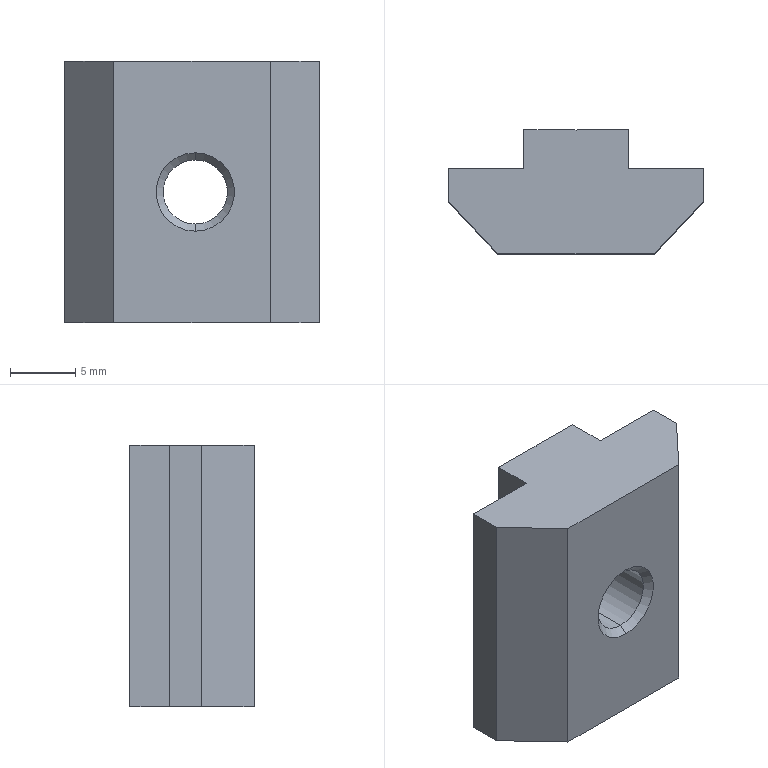Part | SolidWorks | features BaseBody 1 | 1 solid | 23 faces | box 19.5 x 9.5 x 20 mm | volume 2530 mm3 | plane 17 | cone 4 | cylinder 2 | commonest cylinder face diameters 4.917 x2
STEP:
#1=CARTESIAN_POINT('',(10.,0.5415,-7.542));
#2=VERTEX_POINT('',#1);
#3=CARTESIAN_POINT('',(10.,0.5415,-12.458));
#4=VERTEX_POINT('',#3);
#5=CARTESIAN_POINT('',(10.,0.5415,-10.));
#6=DIRECTION('',(0.,-1.,0.));
#7=DIRECTION('',(0.,0.,-1.));
#8=AXIS2_PLACEMENT_3D('',#5,#6,#7);
#9=CIRCLE('',#8,2.458);
#10=EDGE_CURVE('',#2,#4,#9,.T.);
#11=ORIENTED_EDGE('',*,*,#10,.F.);
#12=CARTESIAN_POINT('',(10.,0.,-7.));
#13=VERTEX_POINT('',#12);
#14=CARTESIAN_POINT('',(10.,0.,-7.));
#15=DIRECTION('',(0.,-0.7071,0.7071));
#16=VECTOR('',#15,1000.);
#17=LINE('',#14,#16);
#18=EDGE_CURVE('',#2,#13,#17,.T.);
#19=ORIENTED_EDGE('',*,*,#18,.T.);
#20=CARTESIAN_POINT('',(10.,0.,-13.));
#21=VERTEX_POINT('',#20);
#22=CARTESIAN_POINT('',(10.,0.,-10.));
#23=DIRECTION('',(0.,1.,0.));
#24=DIRECTION('',(0.,0.,-1.));
#25=AXIS2_PLACEMENT_3D('',#22,#23,#24);
#26=CIRCLE('',#25,3.);
#27=EDGE_CURVE('',#21,#13,#26,.T.);
#28=ORIENTED_EDGE('',*,*,#27,.F.);
#29=CARTESIAN_POINT('',(10.,0.,-13.));
#30=DIRECTION('',(0.,-0.7071,-0.7071));
#31=VECTOR('',#30,1000.);
#32=LINE('',#29,#31);
#33=EDGE_CURVE('',#4,#21,#32,.T.);
#34=ORIENTED_EDGE('',*,*,#33,.F.);
#35=EDGE_LOOP('',(#11,#19,#28,#34));
#36=FACE_OUTER_BOUND('',#35,.T.);
#37=CARTESIAN_POINT('',(10.,0.,-10.));
#38=DIRECTION('',(0.,-1.,0.));
#39=DIRECTION('',(0.,0.,-1.));
#40=AXIS2_PLACEMENT_3D('',#37,#38,#39);
#41=CONICAL_SURFACE('',#40,3.,0.7854);
#42=ADVANCED_FACE('',(#36),#41,.F.);
#43=ORIENTED_EDGE('',*,*,#10,.T.);
#44=CARTESIAN_POINT('',(10.,8.959,-12.459));
#45=VERTEX_POINT('',#44);
#46=CARTESIAN_POINT('',(10.,0.,-12.459));
#47=DIRECTION('',(0.,1.,0.));
#48=VECTOR('',#47,1000.);
#49=LINE('',#46,#48);
#50=EDGE_CURVE('',#4,#45,#49,.T.);
#51=ORIENTED_EDGE('',*,*,#50,.T.);
#52=CARTESIAN_POINT('',(10.,8.959,-7.542));
#53=VERTEX_POINT('',#52);
#54=CARTESIAN_POINT('',(10.,8.959,-10.));
#55=DIRECTION('',(0.,-1.,0.));
#56=DIRECTION('',(0.,0.,1.));
#57=AXIS2_PLACEMENT_3D('',#54,#55,#56);
#58=CIRCLE('',#57,2.458);
#59=EDGE_CURVE('',#53,#45,#58,.T.);
#60=ORIENTED_EDGE('',*,*,#59,.F.);
#61=CARTESIAN_POINT('',(10.,0.,-7.542));
#62=DIRECTION('',(0.,1.,0.));
#63=VECTOR('',#62,1000.);
#64=LINE('',#61,#63);
#65=EDGE_CURVE('',#2,#53,#64,.T.);
#66=ORIENTED_EDGE('',*,*,#65,.F.);
#67=EDGE_LOOP('',(#43,#51,#60,#66));
#68=FACE_OUTER_BOUND('',#67,.T.);
#69=CARTESIAN_POINT('',(10.,0.,-10.));
#70=DIRECTION('',(0.,1.,0.));
#71=DIRECTION('',(0.,0.,1.));
#72=AXIS2_PLACEMENT_3D('',#69,#70,#71);
#73=CYLINDRICAL_SURFACE('',#72,2.458);
#74=ADVANCED_FACE('',(#68),#73,.F.);
#75=ORIENTED_EDGE('',*,*,#59,.T.);
#76=CARTESIAN_POINT('',(10.,9.5,-13.));
#77=VERTEX_POINT('',#76);
#78=CARTESIAN_POINT('',(10.,9.5,-13.));
#79=DIRECTION('',(0.,0.7071,-0.7071));
#80=VECTOR('',#79,1000.);
#81=LINE('',#78,#80);
#82=EDGE_CURVE('',#45,#77,#81,.T.);
#83=ORIENTED_EDGE('',*,*,#82,.T.);
#84=CARTESIAN_POINT('',(9.85,9.5,-12.996));
#85=VERTEX_POINT('',#84);
#86=CARTESIAN_POINT('',(10.,9.5,-10.));
#87=DIRECTION('',(0.,-1.,0.));
#88=DIRECTION('',(0.,0.,1.));
#89=AXIS2_PLACEMENT_3D('',#86,#87,#88);
#90=CIRCLE('',#89,3.);
#91=EDGE_CURVE('',#85,#77,#90,.T.);
#92=ORIENTED_EDGE('',*,*,#91,.F.);
#93=CARTESIAN_POINT('',(9.75,9.42,-12.909));
#94=VERTEX_POINT('',#93);
#95=CARTESIAN_POINT('',(9.75,9.42,-12.909));
#96=CARTESIAN_POINT('',(9.783,9.446,-12.938));
#97=CARTESIAN_POINT('',(9.816,9.473,-12.967));
#98=CARTESIAN_POINT('',(9.85,9.5,-12.996));
#99=(BOUNDED_CURVE()B_SPLINE_CURVE(3,(#95,#96,#97,#98),.UNSPECIFIED.,.F.,.F.)B_SPLINE_CURVE_WITH_KNOTS((4,4),(3.735,3.756),.UNSPECIFIED.)CURVE()GEOMETRIC_REPRESENTATION_ITEM()RATIONAL_B_SPLINE_CURVE((1.,1.,1.,1.))REPRESENTATION_ITEM(''));
#100=EDGE_CURVE('',#94,#85,#99,.T.);
#101=ORIENTED_EDGE('',*,*,#100,.F.);
#102=CARTESIAN_POINT('',(9.65,9.5,-12.98));
#103=VERTEX_POINT('',#102);
#104=CARTESIAN_POINT('',(9.65,9.5,-12.98));
#105=CARTESIAN_POINT('',(9.684,9.473,-12.956));
#106=CARTESIAN_POINT('',(9.717,9.446,-12.933));
#107=CARTESIAN_POINT('',(9.75,9.42,-12.909));
#108=(BOUNDED_CURVE()B_SPLINE_CURVE(3,(#104,#105,#106,#107),.UNSPECIFIED.,.F.,.F.)B_SPLINE_CURVE_WITH_KNOTS((4,4),(2.424,2.445),.UNSPECIFIED.)CURVE()GEOMETRIC_REPRESENTATION_ITEM()RATIONAL_B_SPLINE_CURVE((1.,1.,1.,1.))REPRESENTATION_ITEM(''));
#109=EDGE_CURVE('',#103,#94,#108,.T.);
#110=ORIENTED_EDGE('',*,*,#109,.F.);
#111=CARTESIAN_POINT('',(9.65,9.5,-7.02));
#112=VERTEX_POINT('',#111);
#113=CARTESIAN_POINT('',(10.,9.5,-10.));
#114=DIRECTION('',(0.,-1.,0.));
#115=DIRECTION('',(0.,0.,1.));
#116=AXIS2_PLACEMENT_3D('',#113,#114,#115);
#117=CIRCLE('',#116,3.);
#118=EDGE_CURVE('',#112,#103,#117,.T.);
#119=ORIENTED_EDGE('',*,*,#118,.F.);
#120=CARTESIAN_POINT('',(9.75,9.42,-7.091));
#121=VERTEX_POINT('',#120);
#122=CARTESIAN_POINT('',(9.75,9.42,-7.091));
#123=CARTESIAN_POINT('',(9.717,9.446,-7.067));
#124=CARTESIAN_POINT('',(9.684,9.473,-7.044));
#125=CARTESIAN_POINT('',(9.65,9.5,-7.02));
#126=(BOUNDED_CURVE()B_SPLINE_CURVE(3,(#122,#123,#124,#125),.UNSPECIFIED.,.F.,.F.)B_SPLINE_CURVE_WITH_KNOTS((4,4),(3.838,3.859),.UNSPECIFIED.)CURVE()GEOMETRIC_REPRESENTATION_ITEM()RATIONAL_B_SPLINE_CURVE((1.,1.,1.,1.))REPRESENTATION_ITEM(''));
#127=EDGE_CURVE('',#121,#112,#126,.T.);
#128=ORIENTED_EDGE('',*,*,#127,.F.);
#129=CARTESIAN_POINT('',(9.85,9.5,-7.004));
#130=VERTEX_POINT('',#129);
#131=CARTESIAN_POINT('',(9.85,9.5,-7.004));
#132=CARTESIAN_POINT('',(9.816,9.473,-7.033));
#133=CARTESIAN_POINT('',(9.783,9.446,-7.062));
#134=CARTESIAN_POINT('',(9.75,9.42,-7.091));
#135=(BOUNDED_CURVE()B_SPLINE_CURVE(3,(#131,#132,#133,#134),.UNSPECIFIED.,.F.,.F.)B_SPLINE_CURVE_WITH_KNOTS((4,4),(2.528,2.548),.UNSPECIFIED.)CURVE()GEOMETRIC_REPRESENTATION_ITEM()RATIONAL_B_SPLINE_CURVE((1.,1.,1.,1.))REPRESENTATION_ITEM(''));
#136=EDGE_CURVE('',#130,#121,#135,.T.);
#137=ORIENTED_EDGE('',*,*,#136,.F.);
#138=CARTESIAN_POINT('',(10.,9.5,-7.));
#139=VERTEX_POINT('',#138);
#140=CARTESIAN_POINT('',(10.,9.5,-10.));
#141=DIRECTION('',(0.,-1.,0.));
#142=DIRECTION('',(0.,0.,1.));
#143=AXIS2_PLACEMENT_3D('',#140,#141,#142);
#144=CIRCLE('',#143,3.);
#145=EDGE_CURVE('',#139,#130,#144,.T.);
#146=ORIENTED_EDGE('',*,*,#145,.F.);
#147=CARTESIAN_POINT('',(10.,9.5,-7.));
#148=DIRECTION('',(0.,0.7071,0.7071));
#149=VECTOR('',#148,1000.);
#150=LINE('',#147,#149);
#151=EDGE_CURVE('',#53,#139,#150,.T.);
#152=ORIENTED_EDGE('',*,*,#151,.F.);
#153=EDGE_LOOP('',(#75,#83,#92,#101,#110,#119,#128,#137,#146,#152));
#154=FACE_OUTER_BOUND('',#153,.T.);
#155=CARTESIAN_POINT('',(10.,9.5,-10.));
#156=DIRECTION('',(0.,1.,0.));
#157=DIRECTION('',(0.,0.,1.));
#158=AXIS2_PLACEMENT_3D('',#155,#156,#157);
#159=CONICAL_SURFACE('',#158,3.,0.7854);
#160=ADVANCED_FACE('',(#154),#159,.F.);
#161=CARTESIAN_POINT('',(15.75,0.,0.));
#162=VERTEX_POINT('',#161);
#163=CARTESIAN_POINT('',(3.75,0.,0.));
#164=VERTEX_POINT('',#163);
#165=CARTESIAN_POINT('',(3.75,0.,0.));
#166=DIRECTION('',(-1.,0.,0.));
#167=VECTOR('',#166,1000.);
#168=LINE('',#165,#167);
#169=EDGE_CURVE('',#162,#164,#168,.T.);
#170=ORIENTED_EDGE('',*,*,#169,.T.);
#171=CARTESIAN_POINT('',(3.75,0.,-20.));
#172=VERTEX_POINT('',#171);
#173=CARTESIAN_POINT('',(3.75,0.,-20.));
#174=DIRECTION('',(0.,0.,-1.));
#175=VECTOR('',#174,1000.);
#176=LINE('',#173,#175);
#177=EDGE_CURVE('',#164,#172,#176,.T.);
#178=ORIENTED_EDGE('',*,*,#177,.T.);
#179=CARTESIAN_POINT('',(15.75,0.,-20.));
#180=VERTEX_POINT('',#179);
#181=CARTESIAN_POINT('',(3.75,0.,-20.));
#182=DIRECTION('',(1.,0.,0.));
#183=VECTOR('',#182,1000.);
#184=LINE('',#181,#183);
#185=EDGE_CURVE('',#172,#180,#184,.T.);
#186=ORIENTED_EDGE('',*,*,#185,.T.);
#187=CARTESIAN_POINT('',(15.75,0.,-20.));
#188=DIRECTION('',(0.,0.,1.));
#189=VECTOR('',#188,1000.);
#190=LINE('',#187,#189);
#191=EDGE_CURVE('',#180,#162,#190,.T.);
#192=ORIENTED_EDGE('',*,*,#191,.T.);
#193=EDGE_LOOP('',(#170,#178,#186,#192));
#194=FACE_OUTER_BOUND('',#193,.T.);
#195=ORIENTED_EDGE('',*,*,#27,.T.);
#196=CARTESIAN_POINT('',(10.,0.,-10.));
#197=DIRECTION('',(0.,1.,0.));
#198=DIRECTION('',(0.,0.,-1.));
#199=AXIS2_PLACEMENT_3D('',#196,#197,#198);
#200=CIRCLE('',#199,3.);
#201=EDGE_CURVE('',#13,#21,#200,.T.);
#202=ORIENTED_EDGE('',*,*,#201,.T.);
#203=EDGE_LOOP('',(#195,#202));
#204=FACE_BOUND('',#203,.T.);
#205=CARTESIAN_POINT('',(3.75,0.,-20.));
#206=DIRECTION('',(0.,-1.,0.));
#207=DIRECTION('',(0.,0.,-1.));
#208=AXIS2_PLACEMENT_3D('',#205,#206,#207);
#209=PLANE('',#208);
#210=ADVANCED_FACE('',(#194,#204),#209,.T.);
#211=CARTESIAN_POINT('',(0.,4.,0.));
#212=VERTEX_POINT('',#211);
#213=CARTESIAN_POINT('',(0.,4.,0.));
#214=DIRECTION('',(-0.6839,0.7295,0.));
#215=VECTOR('',#214,1000.);
#216=LINE('',#213,#215);
#217=EDGE_CURVE('',#164,#212,#216,.T.);
#218=ORIENTED_EDGE('',*,*,#217,.T.);
#219=CARTESIAN_POINT('',(0.,4.,-20.));
#220=VERTEX_POINT('',#219);
#221=CARTESIAN_POINT('',(0.,4.,-20.));
#222=DIRECTION('',(0.,0.,-1.));
#223=VECTOR('',#222,1000.);
#224=LINE('',#221,#223);
#225=EDGE_CURVE('',#212,#220,#224,.T.);
#226=ORIENTED_EDGE('',*,*,#225,.T.);
#227=CARTESIAN_POINT('',(0.,4.,-20.));
#228=DIRECTION('',(0.6839,-0.7295,0.));
#229=VECTOR('',#228,1000.);
#230=LINE('',#227,#229);
#231=EDGE_CURVE('',#220,#172,#230,.T.);
#232=ORIENTED_EDGE('',*,*,#231,.T.);
#233=ORIENTED_EDGE('',*,*,#177,.F.);
#234=EDGE_LOOP('',(#218,#226,#232,#233));
#235=FACE_OUTER_BOUND('',#234,.T.);
#236=CARTESIAN_POINT('',(0.,4.,-20.));
#237=DIRECTION('',(-0.7295,-0.6839,0.));
#238=DIRECTION('',(0.6839,-0.7295,0.));
#239=AXIS2_PLACEMENT_3D('',#236,#237,#238);
#240=PLANE('',#239);
#241=ADVANCED_FACE('',(#235),#240,.T.);
#242=CARTESIAN_POINT('',(9.75,9.42,0.));
#243=VERTEX_POINT('',#242);
#244=CARTESIAN_POINT('',(9.85,9.5,0.));
#245=VERTEX_POINT('',#244);
#246=CARTESIAN_POINT('',(9.85,9.5,0.));
#247=DIRECTION('',(0.7809,0.6247,0.));
#248=VECTOR('',#247,1000.);
#249=LINE('',#246,#248);
#250=EDGE_CURVE('',#243,#245,#249,.T.);
#251=ORIENTED_EDGE('',*,*,#250,.F.);
#252=CARTESIAN_POINT('',(9.65,9.5,0.));
#253=VERTEX_POINT('',#252);
#254=CARTESIAN_POINT('',(9.75,9.42,0.));
#255=DIRECTION('',(0.7809,-0.6247,0.));
#256=VECTOR('',#255,1000.);
#257=LINE('',#254,#256);
#258=EDGE_CURVE('',#253,#243,#257,.T.);
#259=ORIENTED_EDGE('',*,*,#258,.F.);
#260=CARTESIAN_POINT('',(5.75,9.5,0.));
#261=VERTEX_POINT('',#260);
#262=CARTESIAN_POINT('',(0.,9.5,0.));
#263=DIRECTION('',(-1.,0.,0.));
#264=VECTOR('',#263,1000.);
#265=LINE('',#262,#264);
#266=EDGE_CURVE('',#253,#261,#265,.T.);
#267=ORIENTED_EDGE('',*,*,#266,.T.);
#268=CARTESIAN_POINT('',(5.75,6.5,0.));
#269=VERTEX_POINT('',#268);
#270=CARTESIAN_POINT('',(5.75,0.,0.));
#271=DIRECTION('',(0.,-1.,0.));
#272=VECTOR('',#271,1000.);
#273=LINE('',#270,#272);
#274=EDGE_CURVE('',#261,#269,#273,.T.);
#275=ORIENTED_EDGE('',*,*,#274,.T.);
#276=CARTESIAN_POINT('',(0.,6.5,0.));
#277=VERTEX_POINT('',#276);
#278=CARTESIAN_POINT('',(0.,6.5,0.));
#279=DIRECTION('',(-1.,0.,0.));
#280=VECTOR('',#279,1000.);
#281=LINE('',#278,#280);
#282=EDGE_CURVE('',#269,#277,#281,.T.);
#283=ORIENTED_EDGE('',*,*,#282,.T.);
#284=CARTESIAN_POINT('',(0.,0.,0.));
#285=DIRECTION('',(0.,-1.,0.));
#286=VECTOR('',#285,1000.);
#287=LINE('',#284,#286);
#288=EDGE_CURVE('',#277,#212,#287,.T.);
#289=ORIENTED_EDGE('',*,*,#288,.T.);
#290=ORIENTED_EDGE('',*,*,#217,.F.);
#291=ORIENTED_EDGE('',*,*,#169,.F.);
#292=CARTESIAN_POINT('',(19.5,4.,0.));
#293=VERTEX_POINT('',#292);
#294=CARTESIAN_POINT('',(15.75,0.,0.));
#295=DIRECTION('',(0.6839,0.7295,0.));
#296=VECTOR('',#295,1000.);
#297=LINE('',#294,#296);
#298=EDGE_CURVE('',#162,#293,#297,.T.);
#299=ORIENTED_EDGE('',*,*,#298,.T.);
#300=CARTESIAN_POINT('',(19.5,6.5,0.));
#301=VERTEX_POINT('',#300);
#302=CARTESIAN_POINT('',(19.5,0.,0.));
#303=DIRECTION('',(0.,1.,0.));
#304=VECTOR('',#303,1000.);
#305=LINE('',#302,#304);
#306=EDGE_CURVE('',#293,#301,#305,.T.);
#307=ORIENTED_EDGE('',*,*,#306,.T.);
#308=CARTESIAN_POINT('',(13.75,6.5,0.));
#309=VERTEX_POINT('',#308);
#310=CARTESIAN_POINT('',(0.,6.5,0.));
#311=DIRECTION('',(-1.,0.,0.));
#312=VECTOR('',#311,1000.);
#313=LINE('',#310,#312);
#314=EDGE_CURVE('',#301,#309,#313,.T.);
#315=ORIENTED_EDGE('',*,*,#314,.T.);
#316=CARTESIAN_POINT('',(13.75,9.5,0.));
#317=VERTEX_POINT('',#316);
#318=CARTESIAN_POINT('',(13.75,0.,0.));
#319=DIRECTION('',(0.,1.,0.));
#320=VECTOR('',#319,1000.);
#321=LINE('',#318,#320);
#322=EDGE_CURVE('',#309,#317,#321,.T.);
#323=ORIENTED_EDGE('',*,*,#322,.T.);
#324=CARTESIAN_POINT('',(0.,9.5,0.));
#325=DIRECTION('',(-1.,0.,0.));
#326=VECTOR('',#325,1000.);
#327=LINE('',#324,#326);
#328=EDGE_CURVE('',#317,#245,#327,.T.);
#329=ORIENTED_EDGE('',*,*,#328,.T.);
#330=EDGE_LOOP('',(#251,#259,#267,#275,#283,#289,#290,#291,#299,#307,#315,#323,#329));
#331=FACE_OUTER_BOUND('',#330,.T.);
#332=CARTESIAN_POINT('',(0.,0.,0.));
#333=DIRECTION('',(0.,0.,1.));
#334=DIRECTION('',(1.,0.,0.));
#335=AXIS2_PLACEMENT_3D('',#332,#333,#334);
#336=PLANE('',#335);
#337=ADVANCED_FACE('',(#331),#336,.T.);
#338=ORIENTED_EDGE('',*,*,#298,.F.);
#339=ORIENTED_EDGE('',*,*,#191,.F.);
#340=CARTESIAN_POINT('',(19.5,4.,-20.));
#341=VERTEX_POINT('',#340);
#342=CARTESIAN_POINT('',(15.75,0.,-20.));
#343=DIRECTION('',(0.6839,0.7295,0.));
#344=VECTOR('',#343,1000.);
#345=LINE('',#342,#344);
#346=EDGE_CURVE('',#180,#341,#345,.T.);
#347=ORIENTED_EDGE('',*,*,#346,.T.);
#348=CARTESIAN_POINT('',(19.5,4.,-20.));
#349=DIRECTION('',(0.,0.,1.));
#350=VECTOR('',#349,1000.);
#351=LINE('',#348,#350);
#352=EDGE_CURVE('',#341,#293,#351,.T.);
#353=ORIENTED_EDGE('',*,*,#352,.T.);
#354=EDGE_LOOP('',(#338,#339,#347,#353));
#355=FACE_OUTER_BOUND('',#354,.T.);
#356=CARTESIAN_POINT('',(15.75,0.,-20.));
#357=DIRECTION('',(0.7295,-0.6839,0.));
#358=DIRECTION('',(0.6839,0.7295,0.));
#359=AXIS2_PLACEMENT_3D('',#356,#357,#358);
#360=PLANE('',#359);
#361=ADVANCED_FACE('',(#355),#360,.T.);
#362=CARTESIAN_POINT('',(9.65,9.5,-20.));
#363=VERTEX_POINT('',#362);
#364=CARTESIAN_POINT('',(5.75,9.5,-20.));
#365=VERTEX_POINT('',#364);
#366=CARTESIAN_POINT('',(0.,9.5,-20.));
#367=DIRECTION('',(-1.,0.,0.));
#368=VECTOR('',#367,1000.);
#369=LINE('',#366,#368);
#370=EDGE_CURVE('',#363,#365,#369,.T.);
#371=ORIENTED_EDGE('',*,*,#370,.F.);
#372=CARTESIAN_POINT('',(9.75,9.42,-20.));
#373=VERTEX_POINT('',#372);
#374=CARTESIAN_POINT('',(9.75,9.42,-20.));
#375=DIRECTION('',(-0.7809,0.6247,0.));
#376=VECTOR('',#375,1000.);
#377=LINE('',#374,#376);
#378=EDGE_CURVE('',#373,#363,#377,.T.);
#379=ORIENTED_EDGE('',*,*,#378,.F.);
#380=CARTESIAN_POINT('',(9.85,9.5,-20.));
#381=VERTEX_POINT('',#380);
#382=CARTESIAN_POINT('',(9.85,9.5,-20.));
#383=DIRECTION('',(-0.7809,-0.6247,0.));
#384=VECTOR('',#383,1000.);
#385=LINE('',#382,#384);
#386=EDGE_CURVE('',#381,#373,#385,.T.);
#387=ORIENTED_EDGE('',*,*,#386,.F.);
#388=CARTESIAN_POINT('',(13.75,9.5,-20.));
#389=VERTEX_POINT('',#388);
#390=CARTESIAN_POINT('',(0.,9.5,-20.));
#391=DIRECTION('',(-1.,0.,0.));
#392=VECTOR('',#391,1000.);
#393=LINE('',#390,#392);
#394=EDGE_CURVE('',#389,#381,#393,.T.);
#395=ORIENTED_EDGE('',*,*,#394,.F.);
#396=CARTESIAN_POINT('',(13.75,6.5,-20.));
#397=VERTEX_POINT('',#396);
#398=CARTESIAN_POINT('',(13.75,0.,-20.));
#399=DIRECTION('',(0.,1.,0.));
#400=VECTOR('',#399,1000.);
#401=LINE('',#398,#400);
#402=EDGE_CURVE('',#397,#389,#401,.T.);
#403=ORIENTED_EDGE('',*,*,#402,.F.);
#404=CARTESIAN_POINT('',(19.5,6.5,-20.));
#405=VERTEX_POINT('',#404);
#406=CARTESIAN_POINT('',(0.,6.5,-20.));
#407=DIRECTION('',(-1.,0.,0.));
#408=VECTOR('',#407,1000.);
#409=LINE('',#406,#408);
#410=EDGE_CURVE('',#405,#397,#409,.T.);
#411=ORIENTED_EDGE('',*,*,#410,.F.);
#412=CARTESIAN_POINT('',(19.5,0.,-20.));
#413=DIRECTION('',(0.,1.,0.));
#414=VECTOR('',#413,1000.);
#415=LINE('',#412,#414);
#416=EDGE_CURVE('',#341,#405,#415,.T.);
#417=ORIENTED_EDGE('',*,*,#416,.F.);
#418=ORIENTED_EDGE('',*,*,#346,.F.);
#419=ORIENTED_EDGE('',*,*,#185,.F.);
#420=ORIENTED_EDGE('',*,*,#231,.F.);
#421=CARTESIAN_POINT('',(0.,6.5,-20.));
#422=VERTEX_POINT('',#421);
#423=CARTESIAN_POINT('',(0.,0.,-20.));
#424=DIRECTION('',(0.,-1.,0.));
#425=VECTOR('',#424,1000.);
#426=LINE('',#423,#425);
#427=EDGE_CURVE('',#422,#220,#426,.T.);
#428=ORIENTED_EDGE('',*,*,#427,.F.);
#429=CARTESIAN_POINT('',(5.75,6.5,-20.));
#430=VERTEX_POINT('',#429);
#431=CARTESIAN_POINT('',(0.,6.5,-20.));
#432=DIRECTION('',(-1.,0.,0.));
#433=VECTOR('',#432,1000.);
#434=LINE('',#431,#433);
#435=EDGE_CURVE('',#430,#422,#434,.T.);
#436=ORIENTED_EDGE('',*,*,#435,.F.);
#437=CARTESIAN_POINT('',(5.75,0.,-20.));
#438=DIRECTION('',(0.,-1.,0.));
#439=VECTOR('',#438,1000.);
#440=LINE('',#437,#439);
#441=EDGE_CURVE('',#365,#430,#440,.T.);
#442=ORIENTED_EDGE('',*,*,#441,.F.);
#443=EDGE_LOOP('',(#371,#379,#387,#395,#403,#411,#417,#418,#419,#420,#428,#436,#442));
#444=FACE_OUTER_BOUND('',#443,.T.);
#445=CARTESIAN_POINT('',(0.,0.,-20.));
#446=DIRECTION('',(0.,0.,1.));
#447=DIRECTION('',(1.,0.,0.));
#448=AXIS2_PLACEMENT_3D('',#445,#446,#447);
#449=PLANE('',#448);
#450=ADVANCED_FACE('',(#444),#449,.F.);
#451=ORIENTED_EDGE('',*,*,#18,.F.);
#452=CARTESIAN_POINT('',(10.,0.5415,-10.));
#453=DIRECTION('',(0.,-1.,0.));
#454=DIRECTION('',(0.,0.,-1.));
#455=AXIS2_PLACEMENT_3D('',#452,#453,#454);
#456=CIRCLE('',#455,2.458);
#457=EDGE_CURVE('',#4,#2,#456,.T.);
#458=ORIENTED_EDGE('',*,*,#457,.F.);
#459=ORIENTED_EDGE('',*,*,#33,.T.);
#460=ORIENTED_EDGE('',*,*,#201,.F.);
#461=EDGE_LOOP('',(#451,#458,#459,#460));
#462=FACE_OUTER_BOUND('',#461,.T.);
#463=CARTESIAN_POINT('',(10.,0.,-10.));
#464=DIRECTION('',(0.,-1.,0.));
#465=DIRECTION('',(0.,0.,-1.));
#466=AXIS2_PLACEMENT_3D('',#463,#464,#465);
#467=CONICAL_SURFACE('',#466,3.,0.7854);
#468=ADVANCED_FACE('',(#462),#467,.F.);
#469=ORIENTED_EDGE('',*,*,#288,.F.);
#470=CARTESIAN_POINT('',(0.,6.5,-20.));
#471=DIRECTION('',(0.,0.,-1.));
#472=VECTOR('',#471,1000.);
#473=LINE('',#470,#472);
#474=EDGE_CURVE('',#277,#422,#473,.T.);
#475=ORIENTED_EDGE('',*,*,#474,.T.);
#476=ORIENTED_EDGE('',*,*,#427,.T.);
#477=ORIENTED_EDGE('',*,*,#225,.F.);
#478=EDGE_LOOP('',(#469,#475,#476,#477));
#479=FACE_OUTER_BOUND('',#478,.T.);
#480=CARTESIAN_POINT('',(0.,6.5,-20.));
#481=DIRECTION('',(-1.,0.,0.));
#482=DIRECTION('',(0.,0.,1.));
#483=AXIS2_PLACEMENT_3D('',#480,#481,#482);
#484=PLANE('',#483);
#485=ADVANCED_FACE('',(#479),#484,.T.);
#486=ORIENTED_EDGE('',*,*,#328,.F.);
#487=CARTESIAN_POINT('',(13.75,9.5,-20.));
#488=DIRECTION('',(0.,0.,-1.));
#489=VECTOR('',#488,1000.);
#490=LINE('',#487,#489);
#491=EDGE_CURVE('',#317,#389,#490,.T.);
#492=ORIENTED_EDGE('',*,*,#491,.T.);
#493=ORIENTED_EDGE('',*,*,#394,.T.);
#494=CARTESIAN_POINT('',(9.85,9.5,-20.));
#495=DIRECTION('',(0.,0.,1.));
#496=VECTOR('',#495,1000.);
#497=LINE('',#494,#496);
#498=EDGE_CURVE('',#381,#85,#497,.T.);
#499=ORIENTED_EDGE('',*,*,#498,.T.);
#500=ORIENTED_EDGE('',*,*,#91,.T.);
#501=CARTESIAN_POINT('',(10.,9.5,-10.));
#502=DIRECTION('',(0.,-1.,0.));
#503=DIRECTION('',(0.,0.,1.));
#504=AXIS2_PLACEMENT_3D('',#501,#502,#503);
#505=CIRCLE('',#504,3.);
#506=EDGE_CURVE('',#77,#139,#505,.T.);
#507=ORIENTED_EDGE('',*,*,#506,.T.);
#508=ORIENTED_EDGE('',*,*,#145,.T.);
#509=CARTESIAN_POINT('',(9.85,9.5,-20.));
#510=DIRECTION('',(0.,0.,1.));
#511=VECTOR('',#510,1000.);
#512=LINE('',#509,#511);
#513=EDGE_CURVE('',#130,#245,#512,.T.);
#514=ORIENTED_EDGE('',*,*,#513,.T.);
#515=EDGE_LOOP('',(#486,#492,#493,#499,#500,#507,#508,#514));
#516=FACE_OUTER_BOUND('',#515,.T.);
#517=CARTESIAN_POINT('',(13.75,9.5,-20.));
#518=DIRECTION('',(0.,1.,0.));
#519=DIRECTION('',(0.,0.,1.));
#520=AXIS2_PLACEMENT_3D('',#517,#518,#519);
#521=PLANE('',#520);
#522=ADVANCED_FACE('',(#516),#521,.T.);
#523=ORIENTED_EDGE('',*,*,#322,.F.);
#524=CARTESIAN_POINT('',(13.75,6.5,-20.));
#525=DIRECTION('',(0.,0.,-1.));
#526=VECTOR('',#525,1000.);
#527=LINE('',#524,#526);
#528=EDGE_CURVE('',#309,#397,#527,.T.);
#529=ORIENTED_EDGE('',*,*,#528,.T.);
#530=ORIENTED_EDGE('',*,*,#402,.T.);
#531=ORIENTED_EDGE('',*,*,#491,.F.);
#532=EDGE_LOOP('',(#523,#529,#530,#531));
#533=FACE_OUTER_BOUND('',#532,.T.);
#534=CARTESIAN_POINT('',(13.75,6.5,-20.));
#535=DIRECTION('',(1.,0.,0.));
#536=DIRECTION('',(0.,0.,-1.));
#537=AXIS2_PLACEMENT_3D('',#534,#535,#536);
#538=PLANE('',#537);
#539=ADVANCED_FACE('',(#533),#538,.T.);
#540=ORIENTED_EDGE('',*,*,#314,.F.);
#541=CARTESIAN_POINT('',(19.5,6.5,-20.));
#542=DIRECTION('',(0.,0.,-1.));
#543=VECTOR('',#542,1000.);
#544=LINE('',#541,#543);
#545=EDGE_CURVE('',#301,#405,#544,.T.);
#546=ORIENTED_EDGE('',*,*,#545,.T.);
#547=ORIENTED_EDGE('',*,*,#410,.T.);
#548=ORIENTED_EDGE('',*,*,#528,.F.);
#549=EDGE_LOOP('',(#540,#546,#547,#548));
#550=FACE_OUTER_BOUND('',#549,.T.);
#551=CARTESIAN_POINT('',(19.5,6.5,-20.));
#552=DIRECTION('',(0.,1.,0.));
#553=DIRECTION('',(0.,0.,1.));
#554=AXIS2_PLACEMENT_3D('',#551,#552,#553);
#555=PLANE('',#554);
#556=ADVANCED_FACE('',(#550),#555,.T.);
#557=ORIENTED_EDGE('',*,*,#306,.F.);
#558=ORIENTED_EDGE('',*,*,#352,.F.);
#559=ORIENTED_EDGE('',*,*,#416,.T.);
#560=ORIENTED_EDGE('',*,*,#545,.F.);
#561=EDGE_LOOP('',(#557,#558,#559,#560));
#562=FACE_OUTER_BOUND('',#561,.T.);
#563=CARTESIAN_POINT('',(19.5,4.,-20.));
#564=DIRECTION('',(1.,0.,0.));
#565=DIRECTION('',(0.,0.,-1.));
#566=AXIS2_PLACEMENT_3D('',#563,#564,#565);
#567=PLANE('',#566);
#568=ADVANCED_FACE('',(#562),#567,.T.);
#569=ORIENTED_EDGE('',*,*,#282,.F.);
#570=CARTESIAN_POINT('',(5.75,6.5,-20.));
#571=DIRECTION('',(0.,0.,-1.));
#572=VECTOR('',#571,1000.);
#573=LINE('',#570,#572);
#574=EDGE_CURVE('',#269,#430,#573,.T.);
#575=ORIENTED_EDGE('',*,*,#574,.T.);
#576=ORIENTED_EDGE('',*,*,#435,.T.);
#577=ORIENTED_EDGE('',*,*,#474,.F.);
#578=EDGE_LOOP('',(#569,#575,#576,#577));
#579=FACE_OUTER_BOUND('',#578,.T.);
#580=CARTESIAN_POINT('',(5.75,6.5,-20.));
#581=DIRECTION('',(0.,1.,0.));
#582=DIRECTION('',(0.,0.,1.));
#583=AXIS2_PLACEMENT_3D('',#580,#581,#582);
#584=PLANE('',#583);
#585=ADVANCED_FACE('',(#579),#584,.T.);
#586=ORIENTED_EDGE('',*,*,#274,.F.);
#587=CARTESIAN_POINT('',(5.75,9.5,-20.));
#588=DIRECTION('',(0.,0.,-1.));
#589=VECTOR('',#588,1000.);
#590=LINE('',#587,#589);
#591=EDGE_CURVE('',#261,#365,#590,.T.);
#592=ORIENTED_EDGE('',*,*,#591,.T.);
#593=ORIENTED_EDGE('',*,*,#441,.T.);
#594=ORIENTED_EDGE('',*,*,#574,.F.);
#595=EDGE_LOOP('',(#586,#592,#593,#594));
#596=FACE_OUTER_BOUND('',#595,.T.);
#597=CARTESIAN_POINT('',(5.75,9.5,-20.));
#598=DIRECTION('',(-1.,0.,0.));
#599=DIRECTION('',(0.,0.,1.));
#600=AXIS2_PLACEMENT_3D('',#597,#598,#599);
#601=PLANE('',#600);
#602=ADVANCED_FACE('',(#596),#601,.T.);
#603=CARTESIAN_POINT('',(9.65,9.5,-20.));
#604=DIRECTION('',(0.,0.,-1.));
#605=VECTOR('',#604,1000.);
#606=LINE('',#603,#605);
#607=EDGE_CURVE('',#103,#363,#606,.T.);
#608=ORIENTED_EDGE('',*,*,#607,.T.);
#609=ORIENTED_EDGE('',*,*,#370,.T.);
#610=ORIENTED_EDGE('',*,*,#591,.F.);
#611=ORIENTED_EDGE('',*,*,#266,.F.);
#612=CARTESIAN_POINT('',(9.65,9.5,-20.));
#613=DIRECTION('',(0.,0.,-1.));
#614=VECTOR('',#613,1000.);
#615=LINE('',#612,#614);
#616=EDGE_CURVE('',#253,#112,#615,.T.);
#617=ORIENTED_EDGE('',*,*,#616,.T.);
#618=ORIENTED_EDGE('',*,*,#118,.T.);
#619=EDGE_LOOP('',(#608,#609,#610,#611,#617,#618));
#620=FACE_OUTER_BOUND('',#619,.T.);
#621=CARTESIAN_POINT('',(9.65,9.5,-20.));
#622=DIRECTION('',(0.,1.,0.));
#623=DIRECTION('',(0.,0.,1.));
#624=AXIS2_PLACEMENT_3D('',#621,#622,#623);
#625=PLANE('',#624);
#626=ADVANCED_FACE('',(#620),#625,.T.);
#627=ORIENTED_EDGE('',*,*,#50,.F.);
#628=ORIENTED_EDGE('',*,*,#457,.T.);
#629=ORIENTED_EDGE('',*,*,#65,.T.);
#630=CARTESIAN_POINT('',(10.,8.959,-10.));
#631=DIRECTION('',(0.,-1.,0.));
#632=DIRECTION('',(0.,0.,1.));
#633=AXIS2_PLACEMENT_3D('',#630,#631,#632);
#634=CIRCLE('',#633,2.458);
#635=EDGE_CURVE('',#45,#53,#634,.T.);
#636=ORIENTED_EDGE('',*,*,#635,.F.);
#637=EDGE_LOOP('',(#627,#628,#629,#636));
#638=FACE_OUTER_BOUND('',#637,.T.);
#639=CARTESIAN_POINT('',(10.,0.,-10.));
#640=DIRECTION('',(0.,1.,0.));
#641=DIRECTION('',(0.,0.,1.));
#642=AXIS2_PLACEMENT_3D('',#639,#640,#641);
#643=CYLINDRICAL_SURFACE('',#642,2.458);
#644=ADVANCED_FACE('',(#638),#643,.F.);
#645=ORIENTED_EDGE('',*,*,#513,.F.);
#646=ORIENTED_EDGE('',*,*,#136,.T.);
#647=CARTESIAN_POINT('',(9.75,9.42,-20.));
#648=DIRECTION('',(0.,0.,1.));
#649=VECTOR('',#648,1000.);
#650=LINE('',#647,#649);
#651=EDGE_CURVE('',#121,#243,#650,.T.);
#652=ORIENTED_EDGE('',*,*,#651,.T.);
#653=ORIENTED_EDGE('',*,*,#250,.T.);
#654=EDGE_LOOP('',(#645,#646,#652,#653));
#655=FACE_OUTER_BOUND('',#654,.T.);
#656=CARTESIAN_POINT('',(9.85,9.5,-20.));
#657=DIRECTION('',(-0.6247,0.7809,0.));
#658=DIRECTION('',(-0.7809,-0.6247,0.));
#659=AXIS2_PLACEMENT_3D('',#656,#657,#658);
#660=PLANE('',#659);
#661=ADVANCED_FACE('',(#655),#660,.T.);
#662=ORIENTED_EDGE('',*,*,#82,.F.);
#663=ORIENTED_EDGE('',*,*,#635,.T.);
#664=ORIENTED_EDGE('',*,*,#151,.T.);
#665=ORIENTED_EDGE('',*,*,#506,.F.);
#666=EDGE_LOOP('',(#662,#663,#664,#665));
#667=FACE_OUTER_BOUND('',#666,.T.);
#668=CARTESIAN_POINT('',(10.,9.5,-10.));
#669=DIRECTION('',(0.,1.,0.));
#670=DIRECTION('',(0.,0.,1.));
#671=AXIS2_PLACEMENT_3D('',#668,#669,#670);
#672=CONICAL_SURFACE('',#671,3.,0.7854);
#673=ADVANCED_FACE('',(#667),#672,.F.);
#674=CARTESIAN_POINT('',(9.75,9.42,-20.));
#675=DIRECTION('',(0.,0.,1.));
#676=VECTOR('',#675,1000.);
#677=LINE('',#674,#676);
#678=EDGE_CURVE('',#373,#94,#677,.T.);
#679=ORIENTED_EDGE('',*,*,#678,.T.);
#680=ORIENTED_EDGE('',*,*,#100,.T.);
#681=ORIENTED_EDGE('',*,*,#498,.F.);
#682=ORIENTED_EDGE('',*,*,#386,.T.);
#683=EDGE_LOOP('',(#679,#680,#681,#682));
#684=FACE_OUTER_BOUND('',#683,.T.);
#685=CARTESIAN_POINT('',(9.85,9.5,-20.));
#686=DIRECTION('',(-0.6247,0.7809,0.));
#687=DIRECTION('',(-0.7809,-0.6247,0.));
#688=AXIS2_PLACEMENT_3D('',#685,#686,#687);
#689=PLANE('',#688);
#690=ADVANCED_FACE('',(#684),#689,.T.);
#691=ORIENTED_EDGE('',*,*,#607,.F.);
#692=ORIENTED_EDGE('',*,*,#109,.T.);
#693=ORIENTED_EDGE('',*,*,#678,.F.);
#694=ORIENTED_EDGE('',*,*,#378,.T.);
#695=EDGE_LOOP('',(#691,#692,#693,#694));
#696=FACE_OUTER_BOUND('',#695,.T.);
#697=CARTESIAN_POINT('',(9.75,9.42,-20.));
#698=DIRECTION('',(0.6247,0.7809,0.));
#699=DIRECTION('',(-0.7809,0.6247,0.));
#700=AXIS2_PLACEMENT_3D('',#697,#698,#699);
#701=PLANE('',#700);
#702=ADVANCED_FACE('',(#696),#701,.T.);
#703=ORIENTED_EDGE('',*,*,#651,.F.);
#704=ORIENTED_EDGE('',*,*,#127,.T.);
#705=ORIENTED_EDGE('',*,*,#616,.F.);
#706=ORIENTED_EDGE('',*,*,#258,.T.);
#707=EDGE_LOOP('',(#703,#704,#705,#706));
#708=FACE_OUTER_BOUND('',#707,.T.);
#709=CARTESIAN_POINT('',(9.75,9.42,-20.));
#710=DIRECTION('',(0.6247,0.7809,0.));
#711=DIRECTION('',(-0.7809,0.6247,0.));
#712=AXIS2_PLACEMENT_3D('',#709,#710,#711);
#713=PLANE('',#712);
#714=ADVANCED_FACE('',(#708),#713,.T.);
#715=CLOSED_SHELL('',(#42,#74,#160,#210,#241,#337,#361,#450,#468,#485,#522,#539,#556,#568,#585,#602,#626,#644,#661,#673,#690,#702,#714));
#716=MANIFOLD_SOLID_BREP('',#715);
#717=CARTESIAN_POINT('',(0.,0.,0.));
#718=DIRECTION('',(0.,0.,1.));
#719=DIRECTION('',(1.,0.,0.));
#720=AXIS2_PLACEMENT_3D('',#717,#718,#719);
#721=(LENGTH_UNIT()NAMED_UNIT(*)SI_UNIT(.MILLI.,.METRE.));
#722=UNCERTAINTY_MEASURE_WITH_UNIT(LENGTH_MEASURE(0.00001),#721,'','');
#723=(NAMED_UNIT(*)PLANE_ANGLE_UNIT()SI_UNIT($,.RADIAN.));
#724=(NAMED_UNIT(*)SI_UNIT($,.STERADIAN.)SOLID_ANGLE_UNIT());
#725=(GEOMETRIC_REPRESENTATION_CONTEXT(3)GLOBAL_UNCERTAINTY_ASSIGNED_CONTEXT((#722))GLOBAL_UNIT_ASSIGNED_CONTEXT((#721,#723,#724))REPRESENTATION_CONTEXT('',''));
#726=ADVANCED_BREP_SHAPE_REPRESENTATION('',(#716,#720),#725);